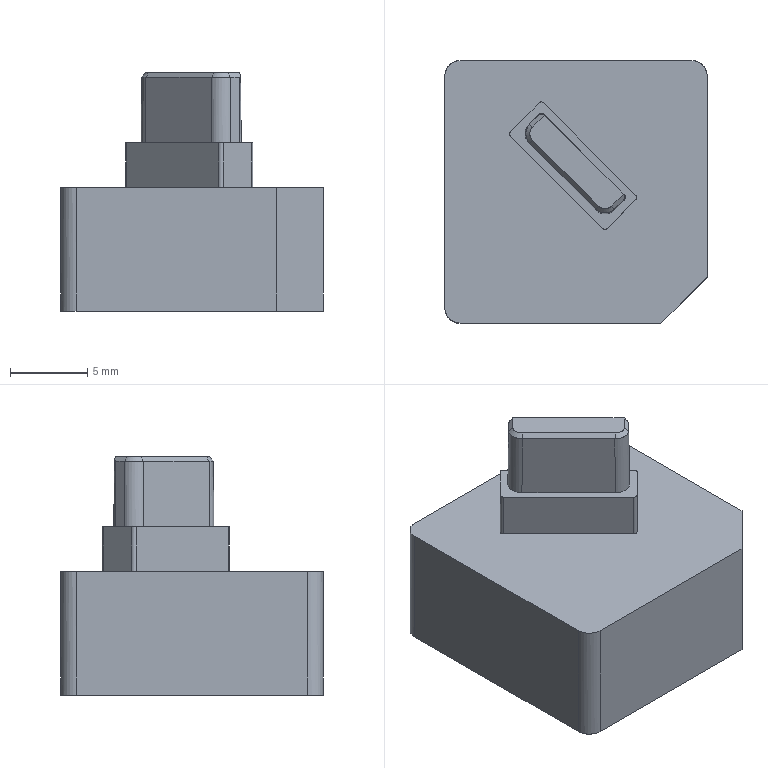NC program | PowerMill | posted with a generic post | part box 17 x 17 x 15.424 mm
Lines 2714 to 3637 of 38437:
N2811 M6
N2812 S8500 M03
N2813 G00 G90 X0.0 Y0.0
N2814 G43 Z11.804 H3
N2815
N2816 G05 P10000 R8
N2817 X-8.0657 Y14.7832
N2818 Z-3.5792
N2819 G01 Z-4.7792 F360.0
N2820 X-5.2685 Y10.3109 F600.0
N2821 X-4.799 Y9.8406
N2822 X-5.0166 Y9.7264
N2823 X-5.2532 Y9.5864
N2824 X-5.4823 Y9.4345
N2825 X-5.5535 Y9.3818
N2826 G03 X-6.0989 Y8.9397 I3.4192 J-4.7753
N2827 G01 X-6.2584 Y8.7866
N2828 X-6.8451 Y8.1998
N2829 X-6.9809 Y8.0591
N2830 G03 X-7.3671 Y7.6075 I6.4461 J-5.9035
N2831 G01 X-7.5264 Y7.3927
N2832 G03 X-7.8915 Y6.8137 I6.9592 J-4.7938
N2833 G01 X-8.0264 Y6.557
N2834 X-8.5725 Y7.1039
N2835 X-8.6231 Y7.143 Z-4.7786
N2836 X-8.6923 Y7.1704 Z-4.7766
N2837 X-8.7755 Y7.1751 Z-4.7728
N2838 X-8.8604 Y7.1495 Z-4.7675
N2839 X-8.9307 Y7.0956 Z-4.7614
N2840 X-8.9754 Y7.0254 Z-4.7559
N2841 X-8.9935 Y6.9533 Z-4.7515
N2842 X-8.9912 Y6.8894 Z-4.7485
N2843 X-8.7766 Y5.5972 Z-4.6964
N2844 X-8.7586 Y5.543 Z-4.6938
N2845 X-8.7163 Y5.4886 Z-4.6901
N2846 X-8.6477 Y5.4504 Z-4.6857
N2847 X-8.5655 Y5.4446 Z-4.6818
N2848 X-8.4921 Y5.4729 Z-4.6794
N2849 X-8.4425 Y5.5208 Z-4.6787
N2850 X-8.417 Y5.572 Z-4.6792
N2851 X-8.3518 Y5.7777 Z-4.683 F360.0
N2852 X-8.2781 Y5.9812 Z-4.6867
N2853 X-8.1393 Y6.3132 Z-4.693
N2854 X-8.022 Y6.5667 Z-4.6979
N2855 X-7.8915 Y6.8137 Z-4.7028
N2856 X-7.7148 Y7.1069 Z-4.7087
N2857 X-7.5264 Y7.3927 Z-4.7147
N2858 X-7.3671 Y7.6075 Z-4.7194
N2859 X-7.1779 Y7.8365 Z-4.7246
N2860 X-6.9809 Y8.0591 Z-4.7298
N2861 X-6.8936 Y8.1496 Z-4.732
N2862 X-6.8451 Y8.1998 Z-4.7332
N2863 X-6.2584 Y8.7866 Z-4.7477
N2864 X-6.0989 Y8.9397 Z-4.7515
N2865 X-5.8328 Y9.1689 Z-4.7576
N2866 X-5.5535 Y9.3818 Z-4.7638
N2867 X-5.4823 Y9.4345 Z-4.7653
N2868 X-5.2532 Y9.5864 Z-4.7701
N2869 X-5.0166 Y9.7264 Z-4.7749
N2870 X-4.799 Y9.8406 Z-4.7792
N2871 X-4.7732 Y9.8541 F600.0
N2872 G02 X-4.2267 Y10.0912 I3.1872 J-6.5982
N2873 G01 X-3.9987 Y10.1711
N2874 X-3.7677 Y10.2417
N2875 X-3.5336 Y10.3013
N2876 X-3.2971 Y10.3504
N2877 X-2.9769 Y10.4001
N2878 X-2.7325 Y10.4282
N2879 X-2.487 Y10.445
N2880 X-2.2411 Y10.4507
N2881 X-1.9951 Y10.445
N2882 G02 X-1.4235 Y10.3888 I-0.3109 J-6.0964
N2883 G01 X-1.1851 Y10.3504
N2884 X-0.9485 Y10.3013
N2885 X-0.7144 Y10.2417
N2886 X-0.4833 Y10.1716
N2887 G02 X0.0415 Y9.9692 I-1.9102 J-5.7349
N2888 G01 X0.2911 Y9.8541
N2889 X0.5345 Y9.7264
N2890 X0.771 Y9.5864
N2891 X1.0001 Y9.4345
N2892 X1.2212 Y9.2711
N2893 G02 X1.7762 Y8.7866 I-3.4803 J-4.548
N2894 G01 X6.9089 Y3.654
N2895 G02 X7.3933 Y3.099 I-4.1138 J-4.0793
N2896 G01 X7.5567 Y2.8779
N2897 X7.7086 Y2.6488
N2898 X7.8486 Y2.4123
N2899 X7.9763 Y2.1689
N2900 X8.1229 Y1.8463
N2901 X8.2134 Y1.6223
N2902 X8.2938 Y1.3945
N2903 X8.3634 Y1.1632
N2904 X8.4236 Y0.9293
N2905 X8.4726 Y0.6927
N2906 G02 X8.5504 Y0.1281 I-7.3291 J-1.2971
N2907 G01 X8.5673 Y-0.1173
N2908 X8.5729 Y-0.3633
N2909 X8.5672 Y-0.6093
N2910 X8.5504 Y-0.8547
N2911 X8.511 Y-1.1808
N2912 X8.4726 Y-1.4193
N2913 X8.423 Y-1.6557
N2914 X8.3639 Y-1.8899
N2915 X8.2938 Y-2.1211
N2916 G02 X8.0915 Y-2.6458 I-5.7719 J1.9246
N2917 G01 X7.9763 Y-2.8955
N2918 X7.8486 Y-3.1388
N2919 G02 X7.5567 Y-3.6045 I-5.4012 J3.0613
N2920 G02 X7.2083 Y-4.0555 I-6.0424 J4.3079
N2921 G01 X7.0614 Y-4.2206
N2922 X6.9088 Y-4.3806
N2923 X6.3221 Y-4.9674
N2924 G02 X5.4491 Y-5.6925 I-4.5806 J4.6263
N2925 G02 X4.6263 Y-6.1732 I-3.5411 J5.1173
N2926 G02 X3.8999 Y-6.474 I-3.0427 J6.3207
N2927 G02 X2.9097 Y-6.7227 I-2.2244 J6.7584
N2928 G02 X1.8786 Y-6.8079 I-1.0993 J7.0244
N2929 G02 X0.8475 Y-6.7228 I0.0673 J7.0991
N2930 G01 X0.6304 Y-6.6821
N2931 G02 X0.0016 Y-6.5197 I1.6675 J7.759
N2932 G02 X-0.5466 Y-6.3184 I1.5504 J5.0691
N2933 G01 X-0.9317 Y-6.1442
N2934 X-1.1787 Y-6.0138
N2935 X-1.5353 Y-5.797
N2936 X-1.7577 Y-5.6486
N2937 X-1.9725 Y-5.4893
N2938 X-2.179 Y-5.3196
N2939 G02 X-2.5649 Y-4.9674 I4.3393 J5.1405
N2940 G01 X-6.8451 Y-0.6871
N2941 G02 X-7.324 Y-0.1471 I4.8402 J4.775
N2942 G01 X-7.3671 Y-0.0947
N2943 X-7.5264 Y0.12
N2944 X-7.7485 Y0.4591
N2945 X-7.8916 Y0.699
N2946 X-8.0219 Y0.9461
N2947 G02 X-8.278 Y1.5316 I8.0833 J3.8844
N2948 G02 X-8.4743 Y2.1502 I5.2769 J2.0145
N2949 G02 X-8.6005 Y2.7253 I6.3371 J1.6924
N2950 G01 X-8.6323 Y2.9438
N2951 X-8.6616 Y3.2386
N2952 X-8.6811 Y3.5341
N2953 G02 X-8.6673 Y4.2006 I5.5123 J0.2194
N2954 G02 X-8.6005 Y4.7875 I6.5427 J-0.4475
N2955 G01 X-8.5598 Y5.0046
N2956 X-8.493 Y5.2891
N2957 X-8.4172 Y5.5713
N2958 X-8.3518 Y5.7777
N2959 X-8.2781 Y5.9812
N2960 X-8.1393 Y6.3132
N2961 X-8.022 Y6.5667
N2962 X-7.8915 Y6.8137
N2963 G02 X-7.5264 Y7.3927 I7.3243 J-4.2148
N2964 G01 X-7.3671 Y7.6075
N2965 G02 X-6.9809 Y8.0591 I6.8323 J-5.4519
N2966 G01 X-6.8451 Y8.1998
N2967 X-6.2584 Y8.7866
N2968 X-6.0989 Y8.9397
N2969 G02 X-5.5535 Y9.3818 I3.9646 J-4.3332
N2970 G01 X-5.4823 Y9.4345
N2971 X-5.2532 Y9.5864
N2972 X-5.0166 Y9.7264
N2973 X-4.799 Y9.8406
N2974 G00 Z4.0043
N2975 G01 X3.0661 Y14.2969 F10000.0
N2976 G00 Z0.9343
N2977 G01 Z-0.2657 F360.0
N2978 X0.5632 Y9.6535 F600.0
N2979 X-7.2083 Y0.2072
N2980 X-7.0497 Y-0.003
N2981 X-6.959 Y-0.1119
N2982 X-6.7756 Y-0.3195
N2983 X-6.6427 Y-0.4589
N2984 X-4.042 Y-3.0597
N2985 X3.9092 Y6.6051
N2986 X6.8568 Y3.6575
N2987 X7.0247 Y3.4818
N2988 X7.1116 Y3.3821
N2989 X-0.5818 Y-5.9694
N2990 G00 Z11.804
N2991 G05 P0
N2992 (---------------)
N2993 ( END TOOLPATH : 精公基准台01-平坦面平行-D10 )
N2994 (---------------)
N2995 ( START TOOLPATH : 精公基准台01-基准面偏置-D10 )
N2996 (---------------)
N2997 G00 X0.0 Y0.0 Z9.8043
N2998 G05 P10000 R8
N2999 X-2.416 Y19.16
N3000 Z-6.42
N3001 G01 Z-7.62 F360.0
N3002 Y13.885 F600.0
N3003 X-2.3664 Y11.1955
N3004 X-2.2082 Y11.197
N3005 X-1.9575 Y11.1912
N3006 X-1.7074 Y11.1736
N3007 X-1.4584 Y11.1445
N3008 X-1.211 Y11.1038
N3009 X-0.9657 Y11.0516
N3010 G02 X-0.089 Y10.7655 I-1.4138 J-5.8194
N3011 G01 X0.0933 Y10.6876
N3012 X0.343 Y10.5654
N3013 X0.586 Y10.4303
N3014 X0.8217 Y10.283
N3015 X1.0972 Y10.0883
N3016 X1.3083 Y9.9241
N3017 X1.5109 Y9.7497
N3018 X1.7046 Y9.5654
N3019 X7.6876 Y3.5824
N3020 G02 X8.0366 Y3.1974 I-4.2301 J-4.1857
N3021 G01 X8.2458 Y2.9272
N3022 X8.4052 Y2.6995
N3023 X8.5526 Y2.4638
N3024 G02 X8.8098 Y1.9711 I-5.2941 J-3.0783
N3025 G01 X8.919 Y1.7155
N3026 G02 X9.1102 Y1.1545 I-6.5026 J-2.5295
N3027 G01 X9.1738 Y0.912
N3028 X9.226 Y0.6668
N3029 X9.2667 Y0.4194
N3030 G02 X9.3134 Y-0.0797 I-6.23 J-0.8342
N3031 G01 X9.3192 Y-0.3962
N3032 X9.3125 Y-0.6468
N3033 X9.2959 Y-0.897
N3034 X9.2667 Y-1.146
N3035 G02 X9.1738 Y-1.6386 I-6.0204 J0.8807
N3036 G01 X9.1103 Y-1.8811
N3037 X9.0149 Y-2.1811
N3038 X8.919 Y-2.4421
N3039 X8.8098 Y-2.6977
N3040 X8.6876 Y-2.9473
N3041 X8.5526 Y-3.1903
N3042 X8.4052 Y-3.426
N3043 X8.2105 Y-3.7016
N3044 X8.0464 Y-3.9126
N3045 X7.8719 Y-4.1152
N3046 X7.6876 Y-4.3089
N3047 X5.8243 Y-6.1723
N3048 G02 X5.0422 Y-6.8193 I-3.9561 J3.9854
N3049 G01 X4.9413 Y-6.8899
N3050 X4.7057 Y-7.0372
N3051 X4.4627 Y-7.1723
N3052 X4.213 Y-7.2945
N3053 X3.9574 Y-7.4037
N3054 X3.6357 Y-7.5201
N3055 X3.3964 Y-7.5949
N3056 X3.1539 Y-7.6585
N3057 X2.9087 Y-7.7107
N3058 X2.6613 Y-7.7514
N3059 X2.4123 Y-7.7806
N3060 X2.1622 Y-7.7981
N3061 G02 X1.5951 I-0.2836 J7.0586
N3062 G01 X1.3449 Y-7.7806
N3063 X1.0959 Y-7.7514
N3064 X0.8485 Y-7.7107
N3065 G02 X-0.4123 Y-7.3131 I1.114 J5.7305
N3066 G01 X-0.7054 Y-7.1723
N3067 X-0.9484 Y-7.0372
N3068 X-1.1841 Y-6.8899
N3069 X-1.4119 Y-6.7305
N3070 G02 X-2.0341 Y-6.2036 I3.2683 J4.4904
N3071 G01 X-3.4611 Y-4.7783
N3072 X-6.9847 Y-8.104
N3073 G02 X-7.8085 Y-8.935 I-0.4257 J-0.4018
N3074 G01 X-8.8645 Y-7.9554
N3075 G02 X-8.8836 Y-7.0453 I0.4306 J0.4643
N3076 G02 X-7.9734 Y-7.0565 I0.4497 J-0.4458
N3077 G01 X-6.9847 Y-8.104
N3078 X-3.4611 Y-4.7783
N3079 X-8.0501 Y-0.1893
N3080 X-8.2344 Y0.0044
N3081 X-8.4088 Y0.207
N3082 X-8.573 Y0.4181
N3083 X-8.7677 Y0.6936
N3084 X-8.915 Y0.9293
N3085 X-9.05 Y1.1723
N3086 X-9.1723 Y1.422
N3087 X-9.2815 Y1.6776
N3088 G02 X-9.4727 Y2.2385 I6.7685 J2.6203
N3089 G01 X-9.5363 Y2.4811
N3090 G02 X-9.6758 Y3.4728 I5.3906 J1.2643
N3091 G01 X-9.6817 Y3.7893
N3092 X-9.6758 Y4.0399
N3093 X-9.6583 Y4.2901
N3094 X-9.6292 Y4.5391
N3095 X-9.5885 Y4.7865
N3096 X-9.5363 Y5.0317
N3097 X-9.4727 Y5.2742
N3098 X-9.3774 Y5.5743
N3099 X-9.2815 Y5.8352
N3100 X-9.1723 Y6.0908
N3101 X-9.05 Y6.3404
N3102 X-8.915 Y6.5834
N3103 X-8.7677 Y6.8191
N3104 X-8.573 Y7.0947
N3105 X-8.4088 Y7.3057
N3106 X-8.2344 Y7.5083
N3107 X-8.0501 Y7.702
N3108 X-6.1867 Y9.5654
N3109 X-5.993 Y9.7497
N3110 X-5.7904 Y9.9241
N3111 X-5.5794 Y10.0883
N3112 X-5.4128 Y10.2078
N3113 X-5.2421 Y10.3215
N3114 X-5.0681 Y10.4303
N3115 X-4.8251 Y10.5654
N3116 X-4.5755 Y10.6876
N3117 G02 X-3.9982 Y10.9132 I2.6108 J-5.8286
N3118 G01 X-3.7589 Y10.988
N3119 G02 X-3.2712 Y11.1038 I1.6328 J-5.7936
N3120 G01 X-3.0238 Y11.1445
N3121 X-2.7747 Y11.1736
N3122 X-2.4455 Y11.1937
N3123 X-2.3664 Y11.1955
N3124 X-2.416 Y13.885
N3125 G00 Z9.8043
N3126 G05 P0
N3127 (---------------)
N3128 ( END TOOLPATH : 精公基准台01-基准面偏置-D10 )
N3129 (---------------)
N3130 ( START TOOLPATH : 精公基准台01-外形侧光-D10 )
N3131 (---------------)
N3132 G00 X0.0 Y0.0 Z10.804
N3133 G05 P10000 R8
N3134 X7.5628 Y-4.5318
N3135 Z-6.39
N3136 G01 Z-7.59 F360.0
N3137 G03 X6.5021 Y-4.9711 I-0.0001 J-1.5 F600.0
N3138 G01 X6.4301 Y-5.0431
N3139 X5.5316 Y-5.9414
N3140 G02 X-1.8177 Y-5.8984 I-3.653 J3.718
N3141 G01 X-4.7706 Y-2.9451
N3142 X-7.8427 Y0.1274
N3143 G02 X-7.7239 Y7.5049 I3.7451 J3.6295
N3144 G01 X-5.8585 Y9.3691
N3145 G02 X1.3331 Y9.4104 I3.6174 J-3.7528
N3146 G02 X1.517 Y9.2297 I-4.4299 J-4.695
N3147 G01 X7.4049 Y3.3418
N3148 G02 X8.6552 Y-2.0953 I-3.6635 J-3.7047
N3149 G02 X7.4005 Y-4.0728 I-4.9298 J1.741
N3150 G01 X6.5021 Y-4.9711
N3151 G03 X6.0627 Y-6.0317 I1.0606 J-1.0607
N3152 G01 X7.5062 Y-4.4753
N3153 G03 X6.4455 Y-4.9146 I-0.0001 J-1.5
N3154 G01 X6.3735 Y-4.9865
N3155 X5.4767 Y-5.8832
N3156 G02 X-1.7612 Y-5.8418 I-3.5981 J3.6598
N3157 G01 X-4.7143 Y-2.8887
N3158 X-7.7847 Y0.1826
N3159 G02 X-7.6674 Y7.4484 I3.687 J3.5743
N3160 G01 X-5.8042 Y9.3104
N3161 G02 X1.2779 Y9.3524 I3.5631 J-3.6941
N3162 G02 X1.4605 Y9.1731 I-4.341 J-4.6028
N3163 G01 X7.3476 Y3.286
N3164 G02 X8.5801 Y-2.0675 I-3.6063 J-3.6489
N3165 G02 X7.3439 Y-4.0162 I-4.8542 J1.7129
N3166 G01 X6.4455 Y-4.9146
N3167 G03 X6.0061 Y-5.9752 I1.0606 J-1.0607
N3168 G00 Z10.804
N3169 G05 P0
N3170 (---------------)
N3171 ( END TOOLPATH : 精公基准台01-外形侧光-D10 )
N3172 (---------------)
N3173 ( START TOOLPATH : 精公基准台01-基准台侧光-D10 )
N3174 (---------------)
N3175 G00 X0.0 Y0.0 Z9.8043
N3176 G05 P10000 R8
N3177 X13.4845 Y-14.7708
N3178 Z-14.32
N3179 G01 Z-15.52 F360.0
N3180 G03 X9.9489 Y-11.2353 I-1.7678 J1.7678 F600.0
N3181 G01 X9.1141 Y-12.0701
N3182 X9.1135 Y-12.0707
N3183 X9.1128 Y-12.0714
N3184 X8.9074 Y-12.2678
N3185 X8.906 Y-12.269
N3186 X8.9046 Y-12.2703
N3187 X8.7671 Y-12.39
N3188 X8.7659 Y-12.3911
N3189 X8.7646 Y-12.3921
N3190 X8.5859 Y-12.5352
N3191 X8.5843 Y-12.5365
N3192 X8.5826 Y-12.5378
N3193 X8.3417 Y-12.7108
N3194 X8.3404 Y-12.7117
N3195 X8.3391 Y-12.7126
N3196 X8.2639 Y-12.7623
N3197 X8.2624 Y-12.7633
N3198 X8.2608 Y-12.7643
N3199 X7.9447 Y-12.953
N3200 X7.9428 Y-12.9541
N3201 X7.9409 Y-12.9551
N3202 X7.7936 Y-13.0328
N3203 X7.7923 Y-13.0334
N3204 X7.791 Y-13.034
N3205 X7.6223 Y-13.1154
N3206 X7.6203 Y-13.1163
N3207 X7.6184 Y-13.1172
N3208 X7.3022 Y-13.2495
N3209 X7.2998 Y-13.2505
N3210 X7.2973 Y-13.2514
N3211 X6.9989 Y-13.3538
N3212 X6.9964 Y-13.3546
N3213 X6.9939 Y-13.3553
N3214 X6.66 Y-13.4457
N3215 X6.6574 Y-13.4464
N3216 X6.6548 Y-13.447
N3217 X6.3386 Y-13.5103
N3218 X6.3361 Y-13.5107
N3219 X6.3336 Y-13.5111
N3220 X6.0174 Y-13.5535
N3221 X6.0149 Y-13.5538
N3222 X6.0124 Y-13.5541
N3223 X5.6962 Y-13.5762
N3224 X5.6939 Y-13.5763
N3225 X5.6915 Y-13.5764
N3226 X5.3754 Y-13.58
N3227 X5.3749
N3228 X5.3745
N3229 X-7.5875 Y-13.5792
N3230 X-7.5891
N3231 X-7.5907
N3232 X-7.9069 Y-13.5663
N3233 X-7.909 Y-13.5662
N3234 X-7.9111 Y-13.5661
N3235 X-8.2273 Y-13.5363
N3236 X-8.2294 Y-13.536
N3237 X-8.2315 Y-13.5357
N3238 X-8.5476 Y-13.489
N3239 X-8.5498 Y-13.4887
N3240 X-8.5519 Y-13.4883
N3241 X-8.868 Y-13.424
N3242 X-8.87 Y-13.4236
N3243 X-8.8719 Y-13.4232
N3244 X-9.1361 Y-13.3556
N3245 X-9.1383 Y-13.3551
N3246 X-9.1404 Y-13.3544
N3247 X-9.5084 Y-13.2385
N3248 X-9.5107 Y-13.2377
N3249 X-9.5129 Y-13.2369
N3250 X-9.8291 Y-13.1162
N3251 X-9.8308 Y-13.1155
N3252 X-9.8324 Y-13.1148
N3253 X-10.0152 Y-13.0353
N3254 X-10.0162 Y-13.0349
N3255 X-10.0173 Y-13.0344
N3256 X-10.1507 Y-12.9716
N3257 X-10.1522 Y-12.9708
N3258 X-10.1537 Y-12.9701
N3259 X-10.4698 Y-12.8052
N3260 X-10.4714 Y-12.8044
N3261 X-10.4729 Y-12.8035
N3262 X-10.6255 Y-12.715
N3263 X-10.6266 Y-12.7144
N3264 X-10.6277 Y-12.7137
N3265 X-10.7912 Y-12.612
N3266 X-10.7928 Y-12.611
N3267 X-10.7943 Y-12.6099
N3268 X-11.1054 Y-12.3956
N3269 X-11.1076 Y-12.394
N3270 X-11.1097 Y-12.3924
N3271 X-11.4309 Y-12.1383
N3272 X-11.4322 Y-12.1372
N3273 X-11.4335 Y-12.1362
N3274 X-11.5055 Y-12.0741
N3275 X-11.5065 Y-12.0732
N3276 X-11.5076 Y-12.0722
N3277 X-11.7518 Y-11.846
N3278 X-11.7529 Y-11.845
N3279 X-11.754 Y-11.8439
N3280 X-11.8439 Y-11.754
N3281 X-11.845 Y-11.7529
N3282 X-11.846 Y-11.7517
N3283 X-12.0722 Y-11.5074
N3284 X-12.0733 Y-11.5062
N3285 X-12.0744 Y-11.505
N3286 X-12.1357 Y-11.4332
N3287 X-12.1367 Y-11.4321
N3288 X-12.1376 Y-11.431
N3289 X-12.3886 Y-11.1148
N3290 X-12.3902 Y-11.1127
N3291 X-12.3918 Y-11.1105
N3292 X-12.6097 Y-10.7944
N3293 X-12.6108 Y-10.7928
N3294 X-12.6118 Y-10.7913
N3295 X-12.7137 Y-10.6278
N3296 X-12.7144 Y-10.6266
N3297 X-12.715 Y-10.6255
N3298 X-12.8035 Y-10.4729
N3299 X-12.8043 Y-10.4714
N3300 X-12.8052 Y-10.4698
N3301 X-12.9703 Y-10.1537
N3302 X-12.9713 Y-10.1516
N3303 X-12.9723 Y-10.1495
N3304 X-13.1144 Y-9.8333
N3305 X-13.1153 Y-9.8312
N3306 X-13.1162 Y-9.8291
N3307 X-13.237 Y-9.5129
N3308 X-13.2378 Y-9.5108
N3309 X-13.2385 Y-9.5087
N3310 X-13.3396 Y-9.1926
N3311 X-13.3402 Y-9.1905
N3312 X-13.3408 Y-9.1884
N3313 X-13.4231 Y-8.8722
N3314 X-13.4236 Y-8.87
N3315 X-13.4241 Y-8.8678
N3316 X-13.4876 Y-8.5517
N3317 X-13.488 Y-8.5497
N3318 X-13.4883 Y-8.5478
N3319 X-13.5357 Y-8.2317
N3320 X-13.536 Y-8.2294
N3321 X-13.5363 Y-8.2271
N3322 X-13.5653 Y-7.911
N3323 X-13.5655 Y-7.909
N3324 X-13.5656 Y-7.9071
N3325 X-13.5792 Y-7.5909
N3326 Y-7.5892
N3327 Y-7.5875
N3328 Y7.5875
N3329 Y7.5891
N3330 Y7.5907
N3331 X-13.5663 Y7.9069
N3332 X-13.5662 Y7.909
N3333 X-13.5661 Y7.9111
N3334 X-13.5363 Y8.2273
N3335 X-13.536 Y8.2294
N3336 X-13.5357 Y8.2315
N3337 X-13.489 Y8.5476
N3338 X-13.4887 Y8.5498
N3339 X-13.4883 Y8.5519
N3340 X-13.424 Y8.868
N3341 X-13.4236 Y8.87
N3342 X-13.4232 Y8.8719
N3343 X-13.3556 Y9.1361
N3344 X-13.3551 Y9.1383
N3345 X-13.3544 Y9.1404
N3346 X-13.2385 Y9.5084
N3347 X-13.2377 Y9.5107
N3348 X-13.2369 Y9.5129
N3349 X-13.1162 Y9.8291
N3350 X-13.1155 Y9.8308
N3351 X-13.1148 Y9.8324
N3352 X-13.0353 Y10.0152
N3353 X-13.0349 Y10.0162
N3354 X-13.0344 Y10.0173
N3355 X-12.9716 Y10.1507
N3356 X-12.9708 Y10.1522
N3357 X-12.9701 Y10.1537
N3358 X-12.8052 Y10.4698
N3359 X-12.8044 Y10.4714
N3360 X-12.8035 Y10.4729
N3361 X-12.715 Y10.6255
N3362 X-12.7144 Y10.6266
N3363 X-12.7137 Y10.6277
N3364 X-12.612 Y10.7912
N3365 X-12.611 Y10.7928
N3366 X-12.6099 Y10.7943
N3367 X-12.3956 Y11.1054
N3368 X-12.394 Y11.1076
N3369 X-12.3924 Y11.1097
N3370 X-12.1383 Y11.4309
N3371 X-12.1372 Y11.4322
N3372 X-12.1362 Y11.4335
N3373 X-12.0741 Y11.5055
N3374 X-12.0732 Y11.5065
N3375 X-12.0722 Y11.5076
N3376 X-11.846 Y11.7518
N3377 X-11.845 Y11.7529
N3378 X-11.8439 Y11.754
N3379 X-11.754 Y11.8439
N3380 X-11.7529 Y11.845
N3381 X-11.7517 Y11.846
N3382 X-11.5074 Y12.0722
N3383 X-11.5062 Y12.0733
N3384 X-11.505 Y12.0744
N3385 X-11.4332 Y12.1357
N3386 X-11.4321 Y12.1367
N3387 X-11.431 Y12.1376
N3388 X-11.1148 Y12.3886
N3389 X-11.1127 Y12.3902
N3390 X-11.1105 Y12.3918
N3391 X-10.7944 Y12.6097
N3392 X-10.7928 Y12.6108
N3393 X-10.7913 Y12.6118
N3394 X-10.6278 Y12.7137
N3395 X-10.6266 Y12.7144
N3396 X-10.6255 Y12.715
N3397 X-10.4729 Y12.8035
N3398 X-10.4714 Y12.8043
N3399 X-10.4698 Y12.8052
N3400 X-10.1537 Y12.9703
N3401 X-10.1516 Y12.9713
N3402 X-10.1495 Y12.9723
N3403 X-9.8333 Y13.1144
N3404 X-9.8312 Y13.1153
N3405 X-9.8291 Y13.1162
N3406 X-9.5129 Y13.237
N3407 X-9.5108 Y13.2378
N3408 X-9.5087 Y13.2385
N3409 X-9.1926 Y13.3396
N3410 X-9.1905 Y13.3402
N3411 X-9.1884 Y13.3408
N3412 X-8.8722 Y13.4231
N3413 X-8.87 Y13.4236
N3414 X-8.8678 Y13.4241
N3415 X-8.5517 Y13.4876
N3416 X-8.5497 Y13.488
N3417 X-8.5478 Y13.4883
N3418 X-8.2317 Y13.5357
N3419 X-8.2294 Y13.536
N3420 X-8.2271 Y13.5363
N3421 X-7.911 Y13.5653
N3422 X-7.909 Y13.5655
N3423 X-7.9071 Y13.5656
N3424 X-7.5909 Y13.5792
N3425 X-7.5892
N3426 X-7.5875
N3427 X0.0
N3428 X7.5875
N3429 X7.5891
N3430 X7.5907
N3431 X7.9069 Y13.5663
N3432 X7.909 Y13.5662
N3433 X7.9111 Y13.5661
N3434 X8.2273 Y13.5363
N3435 X8.2294 Y13.536
N3436 X8.2315 Y13.5357
N3437 X8.5476 Y13.489
N3438 X8.5498 Y13.4887
N3439 X8.5519 Y13.4883
N3440 X8.868 Y13.424
N3441 X8.87 Y13.4236
N3442 X8.8719 Y13.4232
N3443 X9.1361 Y13.3556
N3444 X9.1383 Y13.3551
N3445 X9.1404 Y13.3544
N3446 X9.5084 Y13.2385
N3447 X9.5107 Y13.2377
N3448 X9.5129 Y13.2369
N3449 X9.8291 Y13.1162
N3450 X9.8308 Y13.1155
N3451 X9.8324 Y13.1148
N3452 X10.0152 Y13.0353
N3453 X10.0162 Y13.0349
N3454 X10.0173 Y13.0344
N3455 X10.1507 Y12.9716
N3456 X10.1522 Y12.9708
N3457 X10.1537 Y12.9701
N3458 X10.4698 Y12.8052
N3459 X10.4714 Y12.8044
N3460 X10.4729 Y12.8035
N3461 X10.6255 Y12.715
N3462 X10.6266 Y12.7144
N3463 X10.6277 Y12.7137
N3464 X10.7912 Y12.612
N3465 X10.7928 Y12.611
N3466 X10.7943 Y12.6099
N3467 X11.1054 Y12.3956
N3468 X11.1076 Y12.394
N3469 X11.1097 Y12.3924
N3470 X11.4309 Y12.1383
N3471 X11.4322 Y12.1372
N3472 X11.4335 Y12.1362
N3473 X11.5055 Y12.0741
N3474 X11.5065 Y12.0732
N3475 X11.5076 Y12.0722
N3476 X11.7518 Y11.846
N3477 X11.7529 Y11.845
N3478 X11.754 Y11.8439
N3479 X11.8439 Y11.754
N3480 X11.845 Y11.7529
N3481 X11.846 Y11.7517
N3482 X12.0722 Y11.5074
N3483 X12.0733 Y11.5062
N3484 X12.0744 Y11.505
N3485 X12.1357 Y11.4332
N3486 X12.1367 Y11.4321
N3487 X12.1376 Y11.431
N3488 X12.3886 Y11.1148
N3489 X12.3902 Y11.1127
N3490 X12.3918 Y11.1105
N3491 X12.6097 Y10.7944
N3492 X12.6108 Y10.7928
N3493 X12.6118 Y10.7913
N3494 X12.7137 Y10.6278
N3495 X12.7144 Y10.6266
N3496 X12.715 Y10.6255
N3497 X12.8035 Y10.4729
N3498 X12.8043 Y10.4714
N3499 X12.8052 Y10.4698
N3500 X12.9703 Y10.1537
N3501 X12.9713 Y10.1516
N3502 X12.9723 Y10.1495
N3503 X13.1144 Y9.8333
N3504 X13.1153 Y9.8312
N3505 X13.1162 Y9.8291
N3506 X13.237 Y9.5129
N3507 X13.2378 Y9.5108
N3508 X13.2385 Y9.5087
N3509 X13.3396 Y9.1926
N3510 X13.3403 Y9.1905
N3511 X13.3408 Y9.1884
N3512 X13.4231 Y8.8722
N3513 X13.4236 Y8.87
N3514 X13.4241 Y8.8678
N3515 X13.4876 Y8.5517
N3516 X13.488 Y8.5497
N3517 X13.4883 Y8.5478
N3518 X13.5357 Y8.2317
N3519 X13.536 Y8.2294
N3520 X13.5363 Y8.2271
N3521 X13.5653 Y7.911
N3522 X13.5655 Y7.909
N3523 X13.5656 Y7.9071
N3524 X13.5792 Y7.5909
N3525 Y7.5892
N3526 Y7.5875
N3527 X13.58 Y-5.3745
N3528 Y-5.3749
N3529 Y-5.3754
N3530 X13.5764 Y-5.6915
N3531 X13.5763 Y-5.6939
N3532 X13.5762 Y-5.6962
N3533 X13.5541 Y-6.0124
N3534 X13.5538 Y-6.0149
N3535 X13.5535 Y-6.0174
N3536 X13.5111 Y-6.3336
N3537 X13.5107 Y-6.3361
N3538 X13.5103 Y-6.3386
N3539 X13.447 Y-6.6548
N3540 X13.4464 Y-6.6573
N3541 X13.4458 Y-6.6598
N3542 X13.3608 Y-6.976
N3543 X13.3601 Y-6.9785
N3544 X13.3593 Y-6.981
N3545 X13.2514 Y-7.2972
N3546 X13.2505 Y-7.2997
N3547 X13.2495 Y-7.3022
N3548 X13.1172 Y-7.6184
N3549 X13.1163 Y-7.6203
N3550 X13.1154 Y-7.6223
N3551 X13.034 Y-7.791
N3552 X13.0334 Y-7.7923
N3553 X13.0328 Y-7.7936
N3554 X12.9551 Y-7.9409
N3555 X12.9541 Y-7.9428
N3556 X12.953 Y-7.9447
N3557 X12.7643 Y-8.2608
N3558 X12.7633 Y-8.2624
N3559 X12.7623 Y-8.2639
N3560 X12.7126 Y-8.3391
N3561 X12.7117 Y-8.3404
N3562 X12.7108 Y-8.3417
N3563 X12.5378 Y-8.5826
N3564 X12.5365 Y-8.5843
N3565 X12.5352 Y-8.5859
N3566 X12.3921 Y-8.7646
N3567 X12.3911 Y-8.7659
N3568 X12.39 Y-8.7671
N3569 X12.2703 Y-8.9046
N3570 X12.269 Y-8.906
N3571 X12.2678 Y-8.9074
N3572 X12.0714 Y-9.1128
N3573 X12.0707 Y-9.1135
N3574 X12.0701 Y-9.1141
N3575 X9.9489 Y-11.2353
N3576 G03 X13.4845 Y-14.7708 I1.7678 J-1.7677
N3577 G01 X13.4331 Y-14.709
N3578 G03 X9.8976 Y-11.1735 I-1.7678 J1.7677
N3579 G01 X9.0575 Y-12.0135
N3580 X8.8521 Y-12.2099
N3581 X8.7146 Y-12.3297
N3582 X8.5359 Y-12.4728
N3583 X8.295 Y-12.6458
N3584 X8.2198 Y-12.6956
N3585 X7.9036 Y-12.8844
N3586 X7.7563 Y-12.962
N3587 X7.5875 Y-13.0434
N3588 X7.2714 Y-13.1757
N3589 X6.973 Y-13.2781
N3590 X6.6391 Y-13.3685
N3591 X6.3229 Y-13.4318
N3592 X6.0068 Y-13.4743
N3593 X5.6906 Y-13.4964
N3594 X5.3745 Y-13.5
N3595 X-7.2714
N3596 X-7.5875 Y-13.4992
N3597 X-7.9036 Y-13.4864
N3598 X-8.2198 Y-13.4566
N3599 X-8.5359 Y-13.4099
N3600 X-8.8521 Y-13.3456
N3601 X-9.1163 Y-13.2781
N3602 X-9.4844 Y-13.1622
N3603 X-9.8005 Y-13.0415
N3604 X-9.9832 Y-12.962
N3605 X-10.1167 Y-12.8992
N3606 X-10.4328 Y-12.7343
N3607 X-10.5854 Y-12.6458
N3608 X-10.749 Y-12.544
N3609 X-11.06 Y-12.3297
N3610 X-11.3812 Y-12.0756
N3611 X-11.4532 Y-12.0135
N3612 X-11.6974 Y-11.7873
N3613 X-11.7873 Y-11.6974
N3614 X-12.0135 Y-11.4531
N3615 X-12.0749 Y-11.3812
N3616 X-12.3259 Y-11.0651
N3617 X-12.5439 Y-10.749
N3618 X-12.6458 Y-10.5854
N3619 X-12.7343 Y-10.4328
N3620 X-12.8994 Y-10.1167
N3621 X-13.0415 Y-9.8005
N3622 X-13.1623 Y-9.4844
N3623 X-13.2634 Y-9.1682
N3624 X-13.3457 Y-8.8521
N3625 X-13.4092 Y-8.5359
N3626 X-13.4566 Y-8.2198
N3627 X-13.4857 Y-7.9036
N3628 X-13.4992 Y-7.5875
N3629 X-13.5 Y-7.2714
N3630 Y7.2714
N3631 X-13.4992 Y7.5875
N3632 X-13.4864 Y7.9036
N3633 X-13.4566 Y8.2198
N3634 X-13.4099 Y8.5359
N3635 X-13.3456 Y8.8521
N3636 X-13.2781 Y9.1163
N3637 X-13.1622 Y9.4844
N3638 X-13.0415 Y9.8005
N3639 X-12.962 Y9.9832
N3640 X-12.8992 Y10.1167
N3641 X-12.7343 Y10.4328
N3642 X-12.6458 Y10.5854
N3643 X-12.544 Y10.749
N3644 X-12.3297 Y11.06
N3645 X-12.0756 Y11.3812
N3646 X-12.0135 Y11.4532
N3647 X-11.7873 Y11.6974
N3648 X-11.6974 Y11.7873
N3649 X-11.4531 Y12.0135
N3650 X-11.3812 Y12.0749
N3651 X-11.0651 Y12.3259
N3652 X-10.749 Y12.5439
N3653 X-10.5854 Y12.6458
N3654 X-10.4328 Y12.7343
N3655 X-10.1167 Y12.8994
N3656 X-9.8005 Y13.0415
N3657 X-9.4844 Y13.1623
N3658 X-9.1682 Y13.2634
N3659 X-8.8521 Y13.3457
N3660 X-8.5359 Y13.4092
N3661 X-8.2198 Y13.4566
N3662 X-7.9036 Y13.4857
N3663 X-7.5875 Y13.4992
N3664 X-7.2714 Y13.5
N3665 X0.0
N3666 X7.2714
N3667 X7.5875 Y13.4992
N3668 X7.9036 Y13.4864
N3669 X8.2198 Y13.4566
N3670 X8.5359 Y13.4099
N3671 X8.8521 Y13.3456
N3672 X9.1163 Y13.2781
N3673 X9.4844 Y13.1622
N3674 X9.8005 Y13.0415
N3675 X9.9832 Y12.962
N3676 X10.1167 Y12.8992
N3677 X10.4328 Y12.7343
N3678 X10.5854 Y12.6458
N3679 X10.749 Y12.544
N3680 X11.06 Y12.3297
N3681 X11.3812 Y12.0756
N3682 X11.4532 Y12.0135
N3683 X11.6974 Y11.7873
N3684 X11.7873 Y11.6974
N3685 X12.0135 Y11.4531
N3686 X12.0749 Y11.3812
N3687 X12.3259 Y11.0651
N3688 X12.5439 Y10.749
N3689 X12.6458 Y10.5854
N3690 X12.7343 Y10.4328
N3691 X12.8994 Y10.1167
N3692 X13.0415 Y9.8005
N3693 X13.1623 Y9.4844
N3694 X13.2634 Y9.1682
N3695 X13.3457 Y8.8521
N3696 X13.4092 Y8.5359
N3697 X13.4566 Y8.2198
N3698 X13.4857 Y7.9036
N3699 X13.4992 Y7.5875
N3700 X13.5 Y7.2714
N3701 Y-5.3745
N3702 X13.4964 Y-5.6906
N3703 X13.4743 Y-6.0068
N3704 X13.4318 Y-6.3229
N3705 X13.3685 Y-6.6391
N3706 X13.2836 Y-6.9552
N3707 X13.1757 Y-7.2714
N3708 X13.0434 Y-7.5875
N3709 X12.962 Y-7.7563
N3710 X12.8844 Y-7.9036
N3711 X12.6956 Y-8.2198
N3712 X12.6458 Y-8.295
N3713 X12.4728 Y-8.5359
N3714 X12.3297 Y-8.7146
N3715 X12.2099 Y-8.8521
N3716 X12.0135 Y-9.0575
N3717 X9.8976 Y-11.1735
N3718 G03 X13.4331 Y-14.709 I1.7677 J-1.7678
N3719 G00 Z9.8043
N3720 G05 P0
N3721 (---------------)
N3722 ( END TOOLPATH : 精公基准台01-基准台侧光-D10 )
N3723 (---------------)
N3724
N3725 M05
N3726 G53 Z0.0
N3727 (---------------)
N3728 ( START TOOLPATH : 精公精光01-等高-D4 )
N3729 (---------------)
N3730 ( TOOL NO.    :14 )
N3731 ( TOOL TYPE   : ENDMILL)
N3732 ( TOOL ID     : D4_1_1)
N3733 ( TOOL DIA    : 4.0 LENGTH 62.6)
N3734 T14